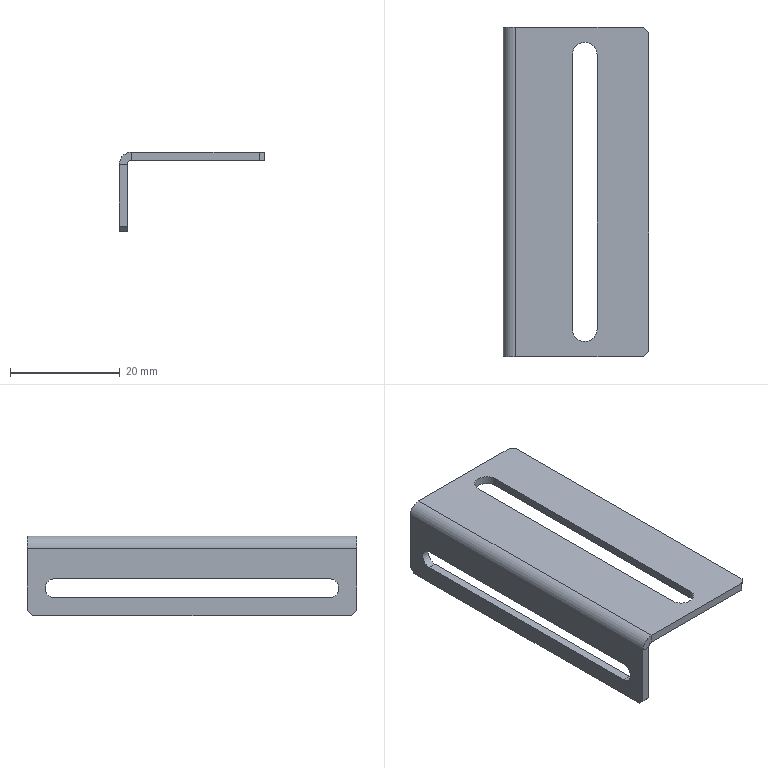Part | SolidWorks | features ICE 2, Chamfer 1, FlatPattern 1, SMBaseFlange 1, SheetMetal 1 | 1 solid | 26 faces | box 26.5 x 60 x 14.5 mm | volume 2856 mm3 | plane 20 | cylinder 6 | commonest cylinder face diameters 3.5 x2 4.5 x2 1.473 x1 4.473 x1
STEP:
#1=CARTESIAN_POINT('',(0.7366,60.,13.));
#2=VERTEX_POINT('',#1);
#3=CARTESIAN_POINT('',(0.7366,60.,14.5));
#4=VERTEX_POINT('',#3);
#5=CARTESIAN_POINT('',(0.7366,60.,13.));
#6=DIRECTION('',(0.,0.,1.));
#7=VECTOR('',#6,1000.);
#8=LINE('',#5,#7);
#9=EDGE_CURVE('',#2,#4,#8,.T.);
#10=ORIENTED_EDGE('',*,*,#9,.F.);
#11=CARTESIAN_POINT('',(0.,60.,12.263));
#12=VERTEX_POINT('',#11);
#13=CARTESIAN_POINT('',(0.7366,60.,12.263));
#14=DIRECTION('',(0.,1.,0.));
#15=DIRECTION('',(0.,0.,-1.));
#16=AXIS2_PLACEMENT_3D('',#13,#14,#15);
#17=CIRCLE('',#16,0.7366);
#18=EDGE_CURVE('',#12,#2,#17,.T.);
#19=ORIENTED_EDGE('',*,*,#18,.F.);
#20=CARTESIAN_POINT('',(-1.5,60.,12.263));
#21=VERTEX_POINT('',#20);
#22=CARTESIAN_POINT('',(-1.5,60.,12.263));
#23=DIRECTION('',(1.,0.,0.));
#24=VECTOR('',#23,1000.);
#25=LINE('',#22,#24);
#26=EDGE_CURVE('',#21,#12,#25,.T.);
#27=ORIENTED_EDGE('',*,*,#26,.F.);
#28=CARTESIAN_POINT('',(0.7366,60.,12.263));
#29=DIRECTION('',(0.,1.,0.));
#30=DIRECTION('',(1.,0.,0.));
#31=AXIS2_PLACEMENT_3D('',#28,#29,#30);
#32=CIRCLE('',#31,2.237);
#33=EDGE_CURVE('',#21,#4,#32,.T.);
#34=ORIENTED_EDGE('',*,*,#33,.T.);
#35=EDGE_LOOP('',(#10,#19,#27,#34));
#36=FACE_OUTER_BOUND('',#35,.T.);
#37=CARTESIAN_POINT('',(0.7366,60.,13.));
#38=DIRECTION('',(0.,1.,0.));
#39=DIRECTION('',(0.,0.,1.));
#40=AXIS2_PLACEMENT_3D('',#37,#38,#39);
#41=PLANE('',#40);
#42=ADVANCED_FACE('',(#36),#41,.T.);
#43=CARTESIAN_POINT('',(24.,60.,14.5));
#44=VERTEX_POINT('',#43);
#45=CARTESIAN_POINT('',(0.,60.,14.5));
#46=DIRECTION('',(1.,0.,0.));
#47=VECTOR('',#46,1000.);
#48=LINE('',#45,#47);
#49=EDGE_CURVE('',#4,#44,#48,.T.);
#50=ORIENTED_EDGE('',*,*,#49,.T.);
#51=CARTESIAN_POINT('',(24.,60.,13.));
#52=VERTEX_POINT('',#51);
#53=CARTESIAN_POINT('',(24.,60.,12.263));
#54=DIRECTION('',(0.,0.,-1.));
#55=VECTOR('',#54,1000.);
#56=LINE('',#53,#55);
#57=EDGE_CURVE('',#44,#52,#56,.T.);
#58=ORIENTED_EDGE('',*,*,#57,.T.);
#59=CARTESIAN_POINT('',(0.,60.,13.));
#60=DIRECTION('',(1.,0.,0.));
#61=VECTOR('',#60,1000.);
#62=LINE('',#59,#61);
#63=EDGE_CURVE('',#2,#52,#62,.T.);
#64=ORIENTED_EDGE('',*,*,#63,.F.);
#65=ORIENTED_EDGE('',*,*,#9,.T.);
#66=EDGE_LOOP('',(#50,#58,#64,#65));
#67=FACE_OUTER_BOUND('',#66,.T.);
#68=CARTESIAN_POINT('',(-1.5,60.,12.263));
#69=DIRECTION('',(0.,1.,0.));
#70=DIRECTION('',(0.,0.,1.));
#71=AXIS2_PLACEMENT_3D('',#68,#69,#70);
#72=PLANE('',#71);
#73=ADVANCED_FACE('',(#67),#72,.T.);
#74=CARTESIAN_POINT('',(0.,0.,12.263));
#75=VERTEX_POINT('',#74);
#76=CARTESIAN_POINT('',(-1.5,0.,12.263));
#77=VERTEX_POINT('',#76);
#78=CARTESIAN_POINT('',(0.,0.,12.263));
#79=DIRECTION('',(-1.,0.,0.));
#80=VECTOR('',#79,1000.);
#81=LINE('',#78,#80);
#82=EDGE_CURVE('',#75,#77,#81,.T.);
#83=ORIENTED_EDGE('',*,*,#82,.F.);
#84=CARTESIAN_POINT('',(0.7366,0.,13.));
#85=VERTEX_POINT('',#84);
#86=CARTESIAN_POINT('',(0.7366,0.,12.263));
#87=DIRECTION('',(0.,1.,0.));
#88=DIRECTION('',(0.,0.,-1.));
#89=AXIS2_PLACEMENT_3D('',#86,#87,#88);
#90=CIRCLE('',#89,0.7366);
#91=EDGE_CURVE('',#75,#85,#90,.T.);
#92=ORIENTED_EDGE('',*,*,#91,.T.);
#93=CARTESIAN_POINT('',(0.7366,0.,14.5));
#94=VERTEX_POINT('',#93);
#95=CARTESIAN_POINT('',(0.7366,0.,14.5));
#96=DIRECTION('',(0.,0.,-1.));
#97=VECTOR('',#96,1000.);
#98=LINE('',#95,#97);
#99=EDGE_CURVE('',#94,#85,#98,.T.);
#100=ORIENTED_EDGE('',*,*,#99,.F.);
#101=CARTESIAN_POINT('',(0.7366,0.,12.263));
#102=DIRECTION('',(0.,1.,0.));
#103=DIRECTION('',(1.,0.,0.));
#104=AXIS2_PLACEMENT_3D('',#101,#102,#103);
#105=CIRCLE('',#104,2.237);
#106=EDGE_CURVE('',#77,#94,#105,.T.);
#107=ORIENTED_EDGE('',*,*,#106,.F.);
#108=EDGE_LOOP('',(#83,#92,#100,#107));
#109=FACE_OUTER_BOUND('',#108,.T.);
#110=CARTESIAN_POINT('',(0.,0.,12.263));
#111=DIRECTION('',(0.,-1.,0.));
#112=DIRECTION('',(0.,0.,-1.));
#113=AXIS2_PLACEMENT_3D('',#110,#111,#112);
#114=PLANE('',#113);
#115=ADVANCED_FACE('',(#109),#114,.T.);
#116=CARTESIAN_POINT('',(-1.5,0.,1.));
#117=VERTEX_POINT('',#116);
#118=CARTESIAN_POINT('',(-1.5,0.,0.));
#119=DIRECTION('',(0.,0.,1.));
#120=VECTOR('',#119,1000.);
#121=LINE('',#118,#120);
#122=EDGE_CURVE('',#117,#77,#121,.T.);
#123=ORIENTED_EDGE('',*,*,#122,.F.);
#124=CARTESIAN_POINT('',(0.,0.,1.));
#125=VERTEX_POINT('',#124);
#126=CARTESIAN_POINT('',(0.7366,0.,1.));
#127=DIRECTION('',(1.,0.,0.));
#128=VECTOR('',#127,1000.);
#129=LINE('',#126,#128);
#130=EDGE_CURVE('',#117,#125,#129,.T.);
#131=ORIENTED_EDGE('',*,*,#130,.T.);
#132=CARTESIAN_POINT('',(0.,0.,0.));
#133=DIRECTION('',(0.,0.,1.));
#134=VECTOR('',#133,1000.);
#135=LINE('',#132,#134);
#136=EDGE_CURVE('',#125,#75,#135,.T.);
#137=ORIENTED_EDGE('',*,*,#136,.T.);
#138=ORIENTED_EDGE('',*,*,#82,.T.);
#139=EDGE_LOOP('',(#123,#131,#137,#138));
#140=FACE_OUTER_BOUND('',#139,.T.);
#141=CARTESIAN_POINT('',(0.7366,0.,14.5));
#142=DIRECTION('',(0.,-1.,0.));
#143=DIRECTION('',(0.,0.,-1.));
#144=AXIS2_PLACEMENT_3D('',#141,#142,#143);
#145=PLANE('',#144);
#146=ADVANCED_FACE('',(#140),#145,.T.);
#147=CARTESIAN_POINT('',(11.1,5.,14.5));
#148=VERTEX_POINT('',#147);
#149=CARTESIAN_POINT('',(11.1,55.,14.5));
#150=VERTEX_POINT('',#149);
#151=CARTESIAN_POINT('',(11.1,55.,14.5));
#152=DIRECTION('',(0.,1.,0.));
#153=VECTOR('',#152,1000.);
#154=LINE('',#151,#153);
#155=EDGE_CURVE('',#148,#150,#154,.T.);
#156=ORIENTED_EDGE('',*,*,#155,.T.);
#157=CARTESIAN_POINT('',(15.6,55.,14.5));
#158=VERTEX_POINT('',#157);
#159=CARTESIAN_POINT('',(13.35,55.,14.5));
#160=DIRECTION('',(0.,0.,-1.));
#161=DIRECTION('',(-1.,0.,0.));
#162=AXIS2_PLACEMENT_3D('',#159,#160,#161);
#163=CIRCLE('',#162,2.25);
#164=EDGE_CURVE('',#150,#158,#163,.T.);
#165=ORIENTED_EDGE('',*,*,#164,.T.);
#166=CARTESIAN_POINT('',(15.6,5.,14.5));
#167=VERTEX_POINT('',#166);
#168=CARTESIAN_POINT('',(15.6,55.,14.5));
#169=DIRECTION('',(0.,-1.,0.));
#170=VECTOR('',#169,1000.);
#171=LINE('',#168,#170);
#172=EDGE_CURVE('',#158,#167,#171,.T.);
#173=ORIENTED_EDGE('',*,*,#172,.T.);
#174=CARTESIAN_POINT('',(13.35,5.,14.5));
#175=DIRECTION('',(0.,0.,-1.));
#176=DIRECTION('',(-1.,0.,0.));
#177=AXIS2_PLACEMENT_3D('',#174,#175,#176);
#178=CIRCLE('',#177,2.25);
#179=EDGE_CURVE('',#167,#148,#178,.T.);
#180=ORIENTED_EDGE('',*,*,#179,.T.);
#181=EDGE_LOOP('',(#156,#165,#173,#180));
#182=FACE_BOUND('',#181,.T.);
#183=CARTESIAN_POINT('',(25.,59.,14.5));
#184=VERTEX_POINT('',#183);
#185=CARTESIAN_POINT('',(25.,1.,14.5));
#186=VERTEX_POINT('',#185);
#187=CARTESIAN_POINT('',(25.,60.,14.5));
#188=DIRECTION('',(0.,-1.,0.));
#189=VECTOR('',#188,1000.);
#190=LINE('',#187,#189);
#191=EDGE_CURVE('',#184,#186,#190,.T.);
#192=ORIENTED_EDGE('',*,*,#191,.F.);
#193=CARTESIAN_POINT('',(25.,59.,14.5));
#194=DIRECTION('',(-0.7071,0.7071,0.));
#195=VECTOR('',#194,1000.);
#196=LINE('',#193,#195);
#197=EDGE_CURVE('',#184,#44,#196,.T.);
#198=ORIENTED_EDGE('',*,*,#197,.T.);
#199=ORIENTED_EDGE('',*,*,#49,.F.);
#200=CARTESIAN_POINT('',(0.7366,60.,14.5));
#201=DIRECTION('',(0.,-1.,0.));
#202=VECTOR('',#201,1000.);
#203=LINE('',#200,#202);
#204=EDGE_CURVE('',#4,#94,#203,.T.);
#205=ORIENTED_EDGE('',*,*,#204,.T.);
#206=CARTESIAN_POINT('',(24.,0.,14.5));
#207=VERTEX_POINT('',#206);
#208=CARTESIAN_POINT('',(0.,0.,14.5));
#209=DIRECTION('',(1.,0.,0.));
#210=VECTOR('',#209,1000.);
#211=LINE('',#208,#210);
#212=EDGE_CURVE('',#94,#207,#211,.T.);
#213=ORIENTED_EDGE('',*,*,#212,.T.);
#214=CARTESIAN_POINT('',(24.,0.,14.5));
#215=DIRECTION('',(0.7071,0.7071,0.));
#216=VECTOR('',#215,1000.);
#217=LINE('',#214,#216);
#218=EDGE_CURVE('',#207,#186,#217,.T.);
#219=ORIENTED_EDGE('',*,*,#218,.T.);
#220=EDGE_LOOP('',(#192,#198,#199,#205,#213,#219));
#221=FACE_OUTER_BOUND('',#220,.T.);
#222=CARTESIAN_POINT('',(0.,60.,14.5));
#223=DIRECTION('',(0.,0.,-1.));
#224=DIRECTION('',(-1.,0.,0.));
#225=AXIS2_PLACEMENT_3D('',#222,#223,#224);
#226=PLANE('',#225);
#227=ADVANCED_FACE('',(#182,#221),#226,.F.);
#228=CARTESIAN_POINT('',(25.,59.,13.));
#229=VERTEX_POINT('',#228);
#230=CARTESIAN_POINT('',(25.,1.,13.));
#231=VERTEX_POINT('',#230);
#232=CARTESIAN_POINT('',(25.,60.,13.));
#233=DIRECTION('',(0.,-1.,0.));
#234=VECTOR('',#233,1000.);
#235=LINE('',#232,#234);
#236=EDGE_CURVE('',#229,#231,#235,.T.);
#237=ORIENTED_EDGE('',*,*,#236,.F.);
#238=CARTESIAN_POINT('',(25.,59.,13.));
#239=DIRECTION('',(0.,0.,1.));
#240=VECTOR('',#239,1000.);
#241=LINE('',#238,#240);
#242=EDGE_CURVE('',#229,#184,#241,.T.);
#243=ORIENTED_EDGE('',*,*,#242,.T.);
#244=ORIENTED_EDGE('',*,*,#191,.T.);
#245=CARTESIAN_POINT('',(25.,1.,13.));
#246=DIRECTION('',(0.,0.,-1.));
#247=VECTOR('',#246,1000.);
#248=LINE('',#245,#247);
#249=EDGE_CURVE('',#186,#231,#248,.T.);
#250=ORIENTED_EDGE('',*,*,#249,.T.);
#251=EDGE_LOOP('',(#237,#243,#244,#250));
#252=FACE_OUTER_BOUND('',#251,.T.);
#253=CARTESIAN_POINT('',(25.,60.,13.));
#254=DIRECTION('',(1.,0.,0.));
#255=DIRECTION('',(0.,0.,-1.));
#256=AXIS2_PLACEMENT_3D('',#253,#254,#255);
#257=PLANE('',#256);
#258=ADVANCED_FACE('',(#252),#257,.T.);
#259=CARTESIAN_POINT('',(11.1,55.,13.));
#260=VERTEX_POINT('',#259);
#261=CARTESIAN_POINT('',(15.6,55.,13.));
#262=VERTEX_POINT('',#261);
#263=CARTESIAN_POINT('',(13.35,55.,13.));
#264=DIRECTION('',(0.,0.,-1.));
#265=DIRECTION('',(-1.,0.,0.));
#266=AXIS2_PLACEMENT_3D('',#263,#264,#265);
#267=CIRCLE('',#266,2.25);
#268=EDGE_CURVE('',#260,#262,#267,.T.);
#269=ORIENTED_EDGE('',*,*,#268,.F.);
#270=CARTESIAN_POINT('',(11.1,5.,13.));
#271=VERTEX_POINT('',#270);
#272=CARTESIAN_POINT('',(11.1,55.,13.));
#273=DIRECTION('',(0.,1.,0.));
#274=VECTOR('',#273,1000.);
#275=LINE('',#272,#274);
#276=EDGE_CURVE('',#271,#260,#275,.T.);
#277=ORIENTED_EDGE('',*,*,#276,.F.);
#278=CARTESIAN_POINT('',(15.6,5.,13.));
#279=VERTEX_POINT('',#278);
#280=CARTESIAN_POINT('',(13.35,5.,13.));
#281=DIRECTION('',(0.,0.,-1.));
#282=DIRECTION('',(-1.,0.,0.));
#283=AXIS2_PLACEMENT_3D('',#280,#281,#282);
#284=CIRCLE('',#283,2.25);
#285=EDGE_CURVE('',#279,#271,#284,.T.);
#286=ORIENTED_EDGE('',*,*,#285,.F.);
#287=CARTESIAN_POINT('',(15.6,55.,13.));
#288=DIRECTION('',(0.,-1.,0.));
#289=VECTOR('',#288,1000.);
#290=LINE('',#287,#289);
#291=EDGE_CURVE('',#262,#279,#290,.T.);
#292=ORIENTED_EDGE('',*,*,#291,.F.);
#293=EDGE_LOOP('',(#269,#277,#286,#292));
#294=FACE_BOUND('',#293,.T.);
#295=ORIENTED_EDGE('',*,*,#63,.T.);
#296=CARTESIAN_POINT('',(12.,72.,13.));
#297=DIRECTION('',(0.7071,-0.7071,0.));
#298=VECTOR('',#297,1000.);
#299=LINE('',#296,#298);
#300=EDGE_CURVE('',#52,#229,#299,.T.);
#301=ORIENTED_EDGE('',*,*,#300,.T.);
#302=ORIENTED_EDGE('',*,*,#236,.T.);
#303=CARTESIAN_POINT('',(24.,0.,13.));
#304=VERTEX_POINT('',#303);
#305=CARTESIAN_POINT('',(42.,18.,13.));
#306=DIRECTION('',(-0.7071,-0.7071,0.));
#307=VECTOR('',#306,1000.);
#308=LINE('',#305,#307);
#309=EDGE_CURVE('',#231,#304,#308,.T.);
#310=ORIENTED_EDGE('',*,*,#309,.T.);
#311=CARTESIAN_POINT('',(0.,0.,13.));
#312=DIRECTION('',(1.,0.,0.));
#313=VECTOR('',#312,1000.);
#314=LINE('',#311,#313);
#315=EDGE_CURVE('',#85,#304,#314,.T.);
#316=ORIENTED_EDGE('',*,*,#315,.F.);
#317=CARTESIAN_POINT('',(0.7366,60.,13.));
#318=DIRECTION('',(0.,-1.,0.));
#319=VECTOR('',#318,1000.);
#320=LINE('',#317,#319);
#321=EDGE_CURVE('',#2,#85,#320,.T.);
#322=ORIENTED_EDGE('',*,*,#321,.F.);
#323=EDGE_LOOP('',(#295,#301,#302,#310,#316,#322));
#324=FACE_OUTER_BOUND('',#323,.T.);
#325=CARTESIAN_POINT('',(0.,60.,13.));
#326=DIRECTION('',(0.,0.,-1.));
#327=DIRECTION('',(-1.,0.,0.));
#328=AXIS2_PLACEMENT_3D('',#325,#326,#327);
#329=PLANE('',#328);
#330=ADVANCED_FACE('',(#294,#324),#329,.T.);
#331=ORIENTED_EDGE('',*,*,#91,.F.);
#332=CARTESIAN_POINT('',(0.,60.,12.263));
#333=DIRECTION('',(0.,-1.,0.));
#334=VECTOR('',#333,1000.);
#335=LINE('',#332,#334);
#336=EDGE_CURVE('',#12,#75,#335,.T.);
#337=ORIENTED_EDGE('',*,*,#336,.F.);
#338=ORIENTED_EDGE('',*,*,#18,.T.);
#339=ORIENTED_EDGE('',*,*,#321,.T.);
#340=EDGE_LOOP('',(#331,#337,#338,#339));
#341=FACE_OUTER_BOUND('',#340,.T.);
#342=CARTESIAN_POINT('',(0.7366,60.,12.263));
#343=DIRECTION('',(0.,-1.,0.));
#344=DIRECTION('',(0.,0.,-1.));
#345=AXIS2_PLACEMENT_3D('',#342,#343,#344);
#346=CYLINDRICAL_SURFACE('',#345,0.7366);
#347=ADVANCED_FACE('',(#341),#346,.F.);
#348=CARTESIAN_POINT('',(0.,55.,3.25));
#349=VERTEX_POINT('',#348);
#350=CARTESIAN_POINT('',(0.,55.,6.75));
#351=VERTEX_POINT('',#350);
#352=CARTESIAN_POINT('',(0.,55.,5.));
#353=DIRECTION('',(1.,0.,0.));
#354=DIRECTION('',(0.,0.,-1.));
#355=AXIS2_PLACEMENT_3D('',#352,#353,#354);
#356=CIRCLE('',#355,1.75);
#357=EDGE_CURVE('',#349,#351,#356,.T.);
#358=ORIENTED_EDGE('',*,*,#357,.F.);
#359=CARTESIAN_POINT('',(0.,5.,3.25));
#360=VERTEX_POINT('',#359);
#361=CARTESIAN_POINT('',(0.,55.,3.25));
#362=DIRECTION('',(0.,1.,0.));
#363=VECTOR('',#362,1000.);
#364=LINE('',#361,#363);
#365=EDGE_CURVE('',#360,#349,#364,.T.);
#366=ORIENTED_EDGE('',*,*,#365,.F.);
#367=CARTESIAN_POINT('',(0.,5.,6.75));
#368=VERTEX_POINT('',#367);
#369=CARTESIAN_POINT('',(0.,5.,5.));
#370=DIRECTION('',(1.,0.,0.));
#371=DIRECTION('',(0.,0.,-1.));
#372=AXIS2_PLACEMENT_3D('',#369,#370,#371);
#373=CIRCLE('',#372,1.75);
#374=EDGE_CURVE('',#368,#360,#373,.T.);
#375=ORIENTED_EDGE('',*,*,#374,.F.);
#376=CARTESIAN_POINT('',(0.,55.,6.75));
#377=DIRECTION('',(0.,-1.,0.));
#378=VECTOR('',#377,1000.);
#379=LINE('',#376,#378);
#380=EDGE_CURVE('',#351,#368,#379,.T.);
#381=ORIENTED_EDGE('',*,*,#380,.F.);
#382=EDGE_LOOP('',(#358,#366,#375,#381));
#383=FACE_BOUND('',#382,.T.);
#384=ORIENTED_EDGE('',*,*,#136,.F.);
#385=CARTESIAN_POINT('',(0.,1.,0.));
#386=VERTEX_POINT('',#385);
#387=CARTESIAN_POINT('',(0.,30.5,-29.5));
#388=DIRECTION('',(0.,0.7071,-0.7071));
#389=VECTOR('',#388,1000.);
#390=LINE('',#387,#389);
#391=EDGE_CURVE('',#125,#386,#390,.T.);
#392=ORIENTED_EDGE('',*,*,#391,.T.);
#393=CARTESIAN_POINT('',(0.,59.,0.));
#394=VERTEX_POINT('',#393);
#395=CARTESIAN_POINT('',(0.,60.,0.));
#396=DIRECTION('',(0.,-1.,0.));
#397=VECTOR('',#396,1000.);
#398=LINE('',#395,#397);
#399=EDGE_CURVE('',#394,#386,#398,.T.);
#400=ORIENTED_EDGE('',*,*,#399,.F.);
#401=CARTESIAN_POINT('',(0.,60.,1.));
#402=VERTEX_POINT('',#401);
#403=CARTESIAN_POINT('',(0.,59.5,0.5));
#404=DIRECTION('',(0.,0.7071,0.7071));
#405=VECTOR('',#404,1000.);
#406=LINE('',#403,#405);
#407=EDGE_CURVE('',#394,#402,#406,.T.);
#408=ORIENTED_EDGE('',*,*,#407,.T.);
#409=CARTESIAN_POINT('',(0.,60.,0.));
#410=DIRECTION('',(0.,0.,1.));
#411=VECTOR('',#410,1000.);
#412=LINE('',#409,#411);
#413=EDGE_CURVE('',#402,#12,#412,.T.);
#414=ORIENTED_EDGE('',*,*,#413,.T.);
#415=ORIENTED_EDGE('',*,*,#336,.T.);
#416=EDGE_LOOP('',(#384,#392,#400,#408,#414,#415));
#417=FACE_OUTER_BOUND('',#416,.T.);
#418=CARTESIAN_POINT('',(0.,60.,0.));
#419=DIRECTION('',(1.,0.,0.));
#420=DIRECTION('',(0.,0.,-1.));
#421=AXIS2_PLACEMENT_3D('',#418,#419,#420);
#422=PLANE('',#421);
#423=ADVANCED_FACE('',(#383,#417),#422,.T.);
#424=ORIENTED_EDGE('',*,*,#399,.T.);
#425=CARTESIAN_POINT('',(-1.5,1.,0.));
#426=VERTEX_POINT('',#425);
#427=CARTESIAN_POINT('',(-1.5,1.,0.));
#428=DIRECTION('',(-1.,0.,0.));
#429=VECTOR('',#428,1000.);
#430=LINE('',#427,#429);
#431=EDGE_CURVE('',#386,#426,#430,.T.);
#432=ORIENTED_EDGE('',*,*,#431,.T.);
#433=CARTESIAN_POINT('',(-1.5,59.,0.));
#434=VERTEX_POINT('',#433);
#435=CARTESIAN_POINT('',(-1.5,60.,0.));
#436=DIRECTION('',(0.,-1.,0.));
#437=VECTOR('',#436,1000.);
#438=LINE('',#435,#437);
#439=EDGE_CURVE('',#434,#426,#438,.T.);
#440=ORIENTED_EDGE('',*,*,#439,.F.);
#441=CARTESIAN_POINT('',(0.,59.,0.));
#442=DIRECTION('',(1.,0.,0.));
#443=VECTOR('',#442,1000.);
#444=LINE('',#441,#443);
#445=EDGE_CURVE('',#434,#394,#444,.T.);
#446=ORIENTED_EDGE('',*,*,#445,.T.);
#447=EDGE_LOOP('',(#424,#432,#440,#446));
#448=FACE_OUTER_BOUND('',#447,.T.);
#449=CARTESIAN_POINT('',(-1.5,60.,0.));
#450=DIRECTION('',(0.,0.,-1.));
#451=DIRECTION('',(-1.,0.,0.));
#452=AXIS2_PLACEMENT_3D('',#449,#450,#451);
#453=PLANE('',#452);
#454=ADVANCED_FACE('',(#448),#453,.T.);
#455=CARTESIAN_POINT('',(-1.5,5.,3.25));
#456=VERTEX_POINT('',#455);
#457=CARTESIAN_POINT('',(-1.5,55.,3.25));
#458=VERTEX_POINT('',#457);
#459=CARTESIAN_POINT('',(-1.5,55.,3.25));
#460=DIRECTION('',(0.,1.,0.));
#461=VECTOR('',#460,1000.);
#462=LINE('',#459,#461);
#463=EDGE_CURVE('',#456,#458,#462,.T.);
#464=ORIENTED_EDGE('',*,*,#463,.T.);
#465=CARTESIAN_POINT('',(-1.5,55.,6.75));
#466=VERTEX_POINT('',#465);
#467=CARTESIAN_POINT('',(-1.5,55.,5.));
#468=DIRECTION('',(1.,0.,0.));
#469=DIRECTION('',(0.,0.,-1.));
#470=AXIS2_PLACEMENT_3D('',#467,#468,#469);
#471=CIRCLE('',#470,1.75);
#472=EDGE_CURVE('',#458,#466,#471,.T.);
#473=ORIENTED_EDGE('',*,*,#472,.T.);
#474=CARTESIAN_POINT('',(-1.5,5.,6.75));
#475=VERTEX_POINT('',#474);
#476=CARTESIAN_POINT('',(-1.5,55.,6.75));
#477=DIRECTION('',(0.,-1.,0.));
#478=VECTOR('',#477,1000.);
#479=LINE('',#476,#478);
#480=EDGE_CURVE('',#466,#475,#479,.T.);
#481=ORIENTED_EDGE('',*,*,#480,.T.);
#482=CARTESIAN_POINT('',(-1.5,5.,5.));
#483=DIRECTION('',(1.,0.,0.));
#484=DIRECTION('',(0.,0.,-1.));
#485=AXIS2_PLACEMENT_3D('',#482,#483,#484);
#486=CIRCLE('',#485,1.75);
#487=EDGE_CURVE('',#475,#456,#486,.T.);
#488=ORIENTED_EDGE('',*,*,#487,.T.);
#489=EDGE_LOOP('',(#464,#473,#481,#488));
#490=FACE_BOUND('',#489,.T.);
#491=ORIENTED_EDGE('',*,*,#439,.T.);
#492=CARTESIAN_POINT('',(-1.5,0.,1.));
#493=DIRECTION('',(0.,-0.7071,0.7071));
#494=VECTOR('',#493,1000.);
#495=LINE('',#492,#494);
#496=EDGE_CURVE('',#426,#117,#495,.T.);
#497=ORIENTED_EDGE('',*,*,#496,.T.);
#498=ORIENTED_EDGE('',*,*,#122,.T.);
#499=CARTESIAN_POINT('',(-1.5,60.,12.263));
#500=DIRECTION('',(0.,-1.,0.));
#501=VECTOR('',#500,1000.);
#502=LINE('',#499,#501);
#503=EDGE_CURVE('',#21,#77,#502,.T.);
#504=ORIENTED_EDGE('',*,*,#503,.F.);
#505=CARTESIAN_POINT('',(-1.5,60.,1.));
#506=VERTEX_POINT('',#505);
#507=CARTESIAN_POINT('',(-1.5,60.,0.));
#508=DIRECTION('',(0.,0.,1.));
#509=VECTOR('',#508,1000.);
#510=LINE('',#507,#509);
#511=EDGE_CURVE('',#506,#21,#510,.T.);
#512=ORIENTED_EDGE('',*,*,#511,.F.);
#513=CARTESIAN_POINT('',(-1.5,59.,0.));
#514=DIRECTION('',(0.,-0.7071,-0.7071));
#515=VECTOR('',#514,1000.);
#516=LINE('',#513,#515);
#517=EDGE_CURVE('',#506,#434,#516,.T.);
#518=ORIENTED_EDGE('',*,*,#517,.T.);
#519=EDGE_LOOP('',(#491,#497,#498,#504,#512,#518));
#520=FACE_OUTER_BOUND('',#519,.T.);
#521=CARTESIAN_POINT('',(-1.5,60.,0.));
#522=DIRECTION('',(1.,0.,0.));
#523=DIRECTION('',(0.,0.,-1.));
#524=AXIS2_PLACEMENT_3D('',#521,#522,#523);
#525=PLANE('',#524);
#526=ADVANCED_FACE('',(#490,#520),#525,.F.);
#527=ORIENTED_EDGE('',*,*,#106,.T.);
#528=ORIENTED_EDGE('',*,*,#204,.F.);
#529=ORIENTED_EDGE('',*,*,#33,.F.);
#530=ORIENTED_EDGE('',*,*,#503,.T.);
#531=EDGE_LOOP('',(#527,#528,#529,#530));
#532=FACE_OUTER_BOUND('',#531,.T.);
#533=CARTESIAN_POINT('',(0.7366,60.,12.263));
#534=DIRECTION('',(0.,-1.,0.));
#535=DIRECTION('',(0.,0.,-1.));
#536=AXIS2_PLACEMENT_3D('',#533,#534,#535);
#537=CYLINDRICAL_SURFACE('',#536,2.237);
#538=ADVANCED_FACE('',(#532),#537,.T.);
#539=ORIENTED_EDGE('',*,*,#413,.F.);
#540=CARTESIAN_POINT('',(-1.5,60.,1.));
#541=DIRECTION('',(-1.,0.,0.));
#542=VECTOR('',#541,1000.);
#543=LINE('',#540,#542);
#544=EDGE_CURVE('',#402,#506,#543,.T.);
#545=ORIENTED_EDGE('',*,*,#544,.T.);
#546=ORIENTED_EDGE('',*,*,#511,.T.);
#547=ORIENTED_EDGE('',*,*,#26,.T.);
#548=EDGE_LOOP('',(#539,#545,#546,#547));
#549=FACE_OUTER_BOUND('',#548,.T.);
#550=CARTESIAN_POINT('',(0.7366,60.,12.263));
#551=DIRECTION('',(0.,-1.,0.));
#552=DIRECTION('',(-1.,0.,0.));
#553=AXIS2_PLACEMENT_3D('',#550,#551,#552);
#554=PLANE('',#553);
#555=ADVANCED_FACE('',(#549),#554,.F.);
#556=ORIENTED_EDGE('',*,*,#315,.T.);
#557=CARTESIAN_POINT('',(24.,0.,12.263));
#558=DIRECTION('',(0.,0.,1.));
#559=VECTOR('',#558,1000.);
#560=LINE('',#557,#559);
#561=EDGE_CURVE('',#304,#207,#560,.T.);
#562=ORIENTED_EDGE('',*,*,#561,.T.);
#563=ORIENTED_EDGE('',*,*,#212,.F.);
#564=ORIENTED_EDGE('',*,*,#99,.T.);
#565=EDGE_LOOP('',(#556,#562,#563,#564));
#566=FACE_OUTER_BOUND('',#565,.T.);
#567=CARTESIAN_POINT('',(0.7366,0.,12.263));
#568=DIRECTION('',(0.,-1.,0.));
#569=DIRECTION('',(-1.,0.,0.));
#570=AXIS2_PLACEMENT_3D('',#567,#568,#569);
#571=PLANE('',#570);
#572=ADVANCED_FACE('',(#566),#571,.T.);
#573=ORIENTED_EDGE('',*,*,#357,.T.);
#574=CARTESIAN_POINT('',(-1.5,55.,6.75));
#575=DIRECTION('',(1.,0.,0.));
#576=VECTOR('',#575,1000.);
#577=LINE('',#574,#576);
#578=EDGE_CURVE('',#466,#351,#577,.T.);
#579=ORIENTED_EDGE('',*,*,#578,.F.);
#580=ORIENTED_EDGE('',*,*,#472,.F.);
#581=CARTESIAN_POINT('',(-1.5,55.,3.25));
#582=DIRECTION('',(1.,0.,0.));
#583=VECTOR('',#582,1000.);
#584=LINE('',#581,#583);
#585=EDGE_CURVE('',#458,#349,#584,.T.);
#586=ORIENTED_EDGE('',*,*,#585,.T.);
#587=EDGE_LOOP('',(#573,#579,#580,#586));
#588=FACE_OUTER_BOUND('',#587,.T.);
#589=CARTESIAN_POINT('',(-1.5,55.,5.));
#590=DIRECTION('',(1.,0.,0.));
#591=DIRECTION('',(0.,0.,-1.));
#592=AXIS2_PLACEMENT_3D('',#589,#590,#591);
#593=CYLINDRICAL_SURFACE('',#592,1.75);
#594=ADVANCED_FACE('',(#588),#593,.F.);
#595=ORIENTED_EDGE('',*,*,#365,.T.);
#596=ORIENTED_EDGE('',*,*,#585,.F.);
#597=ORIENTED_EDGE('',*,*,#463,.F.);
#598=CARTESIAN_POINT('',(-1.5,5.,3.25));
#599=DIRECTION('',(1.,0.,0.));
#600=VECTOR('',#599,1000.);
#601=LINE('',#598,#600);
#602=EDGE_CURVE('',#456,#360,#601,.T.);
#603=ORIENTED_EDGE('',*,*,#602,.T.);
#604=EDGE_LOOP('',(#595,#596,#597,#603));
#605=FACE_OUTER_BOUND('',#604,.T.);
#606=CARTESIAN_POINT('',(-1.5,55.,3.25));
#607=DIRECTION('',(0.,0.,-1.));
#608=DIRECTION('',(-1.,0.,0.));
#609=AXIS2_PLACEMENT_3D('',#606,#607,#608);
#610=PLANE('',#609);
#611=ADVANCED_FACE('',(#605),#610,.F.);
#612=ORIENTED_EDGE('',*,*,#374,.T.);
#613=ORIENTED_EDGE('',*,*,#602,.F.);
#614=ORIENTED_EDGE('',*,*,#487,.F.);
#615=CARTESIAN_POINT('',(-1.5,5.,6.75));
#616=DIRECTION('',(1.,0.,0.));
#617=VECTOR('',#616,1000.);
#618=LINE('',#615,#617);
#619=EDGE_CURVE('',#475,#368,#618,.T.);
#620=ORIENTED_EDGE('',*,*,#619,.T.);
#621=EDGE_LOOP('',(#612,#613,#614,#620));
#622=FACE_OUTER_BOUND('',#621,.T.);
#623=CARTESIAN_POINT('',(-1.5,5.,5.));
#624=DIRECTION('',(1.,0.,0.));
#625=DIRECTION('',(0.,0.,-1.));
#626=AXIS2_PLACEMENT_3D('',#623,#624,#625);
#627=CYLINDRICAL_SURFACE('',#626,1.75);
#628=ADVANCED_FACE('',(#622),#627,.F.);
#629=ORIENTED_EDGE('',*,*,#380,.T.);
#630=ORIENTED_EDGE('',*,*,#619,.F.);
#631=ORIENTED_EDGE('',*,*,#480,.F.);
#632=ORIENTED_EDGE('',*,*,#578,.T.);
#633=EDGE_LOOP('',(#629,#630,#631,#632));
#634=FACE_OUTER_BOUND('',#633,.T.);
#635=CARTESIAN_POINT('',(-1.5,55.,6.75));
#636=DIRECTION('',(0.,0.,1.));
#637=DIRECTION('',(1.,0.,0.));
#638=AXIS2_PLACEMENT_3D('',#635,#636,#637);
#639=PLANE('',#638);
#640=ADVANCED_FACE('',(#634),#639,.F.);
#641=ORIENTED_EDGE('',*,*,#300,.F.);
#642=ORIENTED_EDGE('',*,*,#57,.F.);
#643=ORIENTED_EDGE('',*,*,#197,.F.);
#644=ORIENTED_EDGE('',*,*,#242,.F.);
#645=EDGE_LOOP('',(#641,#642,#643,#644));
#646=FACE_OUTER_BOUND('',#645,.T.);
#647=CARTESIAN_POINT('',(25.,59.,13.));
#648=DIRECTION('',(-0.7071,-0.7071,0.));
#649=DIRECTION('',(0.,0.,1.));
#650=AXIS2_PLACEMENT_3D('',#647,#648,#649);
#651=PLANE('',#650);
#652=ADVANCED_FACE('',(#646),#651,.F.);
#653=ORIENTED_EDGE('',*,*,#309,.F.);
#654=ORIENTED_EDGE('',*,*,#249,.F.);
#655=ORIENTED_EDGE('',*,*,#218,.F.);
#656=ORIENTED_EDGE('',*,*,#561,.F.);
#657=EDGE_LOOP('',(#653,#654,#655,#656));
#658=FACE_OUTER_BOUND('',#657,.T.);
#659=CARTESIAN_POINT('',(24.,0.,12.263));
#660=DIRECTION('',(-0.7071,0.7071,0.));
#661=DIRECTION('',(0.,0.,1.));
#662=AXIS2_PLACEMENT_3D('',#659,#660,#661);
#663=PLANE('',#662);
#664=ADVANCED_FACE('',(#658),#663,.F.);
#665=ORIENTED_EDGE('',*,*,#496,.F.);
#666=ORIENTED_EDGE('',*,*,#431,.F.);
#667=ORIENTED_EDGE('',*,*,#391,.F.);
#668=ORIENTED_EDGE('',*,*,#130,.F.);
#669=EDGE_LOOP('',(#665,#666,#667,#668));
#670=FACE_OUTER_BOUND('',#669,.T.);
#671=CARTESIAN_POINT('',(0.7366,0.,1.));
#672=DIRECTION('',(0.,0.7071,0.7071));
#673=DIRECTION('',(1.,0.,0.));
#674=AXIS2_PLACEMENT_3D('',#671,#672,#673);
#675=PLANE('',#674);
#676=ADVANCED_FACE('',(#670),#675,.F.);
#677=ORIENTED_EDGE('',*,*,#517,.F.);
#678=ORIENTED_EDGE('',*,*,#544,.F.);
#679=ORIENTED_EDGE('',*,*,#407,.F.);
#680=ORIENTED_EDGE('',*,*,#445,.F.);
#681=EDGE_LOOP('',(#677,#678,#679,#680));
#682=FACE_OUTER_BOUND('',#681,.T.);
#683=CARTESIAN_POINT('',(-1.5,59.,0.));
#684=DIRECTION('',(0.,0.7071,-0.7071));
#685=DIRECTION('',(-1.,0.,0.));
#686=AXIS2_PLACEMENT_3D('',#683,#684,#685);
#687=PLANE('',#686);
#688=ADVANCED_FACE('',(#682),#687,.T.);
#689=ORIENTED_EDGE('',*,*,#268,.T.);
#690=CARTESIAN_POINT('',(15.6,55.,14.5));
#691=DIRECTION('',(0.,0.,-1.));
#692=VECTOR('',#691,1000.);
#693=LINE('',#690,#692);
#694=EDGE_CURVE('',#158,#262,#693,.T.);
#695=ORIENTED_EDGE('',*,*,#694,.F.);
#696=ORIENTED_EDGE('',*,*,#164,.F.);
#697=CARTESIAN_POINT('',(11.1,55.,14.5));
#698=DIRECTION('',(0.,0.,-1.));
#699=VECTOR('',#698,1000.);
#700=LINE('',#697,#699);
#701=EDGE_CURVE('',#150,#260,#700,.T.);
#702=ORIENTED_EDGE('',*,*,#701,.T.);
#703=EDGE_LOOP('',(#689,#695,#696,#702));
#704=FACE_OUTER_BOUND('',#703,.T.);
#705=CARTESIAN_POINT('',(13.35,55.,14.5));
#706=DIRECTION('',(0.,0.,-1.));
#707=DIRECTION('',(-1.,0.,0.));
#708=AXIS2_PLACEMENT_3D('',#705,#706,#707);
#709=CYLINDRICAL_SURFACE('',#708,2.25);
#710=ADVANCED_FACE('',(#704),#709,.F.);
#711=ORIENTED_EDGE('',*,*,#276,.T.);
#712=ORIENTED_EDGE('',*,*,#701,.F.);
#713=ORIENTED_EDGE('',*,*,#155,.F.);
#714=CARTESIAN_POINT('',(11.1,5.,14.5));
#715=DIRECTION('',(0.,0.,-1.));
#716=VECTOR('',#715,1000.);
#717=LINE('',#714,#716);
#718=EDGE_CURVE('',#148,#271,#717,.T.);
#719=ORIENTED_EDGE('',*,*,#718,.T.);
#720=EDGE_LOOP('',(#711,#712,#713,#719));
#721=FACE_OUTER_BOUND('',#720,.T.);
#722=CARTESIAN_POINT('',(11.1,55.,14.5));
#723=DIRECTION('',(-1.,0.,0.));
#724=DIRECTION('',(0.,-1.,0.));
#725=AXIS2_PLACEMENT_3D('',#722,#723,#724);
#726=PLANE('',#725);
#727=ADVANCED_FACE('',(#721),#726,.F.);
#728=ORIENTED_EDGE('',*,*,#285,.T.);
#729=ORIENTED_EDGE('',*,*,#718,.F.);
#730=ORIENTED_EDGE('',*,*,#179,.F.);
#731=CARTESIAN_POINT('',(15.6,5.,14.5));
#732=DIRECTION('',(0.,0.,-1.));
#733=VECTOR('',#732,1000.);
#734=LINE('',#731,#733);
#735=EDGE_CURVE('',#167,#279,#734,.T.);
#736=ORIENTED_EDGE('',*,*,#735,.T.);
#737=EDGE_LOOP('',(#728,#729,#730,#736));
#738=FACE_OUTER_BOUND('',#737,.T.);
#739=CARTESIAN_POINT('',(13.35,5.,14.5));
#740=DIRECTION('',(0.,0.,-1.));
#741=DIRECTION('',(-1.,0.,0.));
#742=AXIS2_PLACEMENT_3D('',#739,#740,#741);
#743=CYLINDRICAL_SURFACE('',#742,2.25);
#744=ADVANCED_FACE('',(#738),#743,.F.);
#745=ORIENTED_EDGE('',*,*,#291,.T.);
#746=ORIENTED_EDGE('',*,*,#735,.F.);
#747=ORIENTED_EDGE('',*,*,#172,.F.);
#748=ORIENTED_EDGE('',*,*,#694,.T.);
#749=EDGE_LOOP('',(#745,#746,#747,#748));
#750=FACE_OUTER_BOUND('',#749,.T.);
#751=CARTESIAN_POINT('',(15.6,55.,14.5));
#752=DIRECTION('',(1.,0.,0.));
#753=DIRECTION('',(0.,1.,0.));
#754=AXIS2_PLACEMENT_3D('',#751,#752,#753);
#755=PLANE('',#754);
#756=ADVANCED_FACE('',(#750),#755,.F.);
#757=CLOSED_SHELL('',(#42,#73,#115,#146,#227,#258,#330,#347,#423,#454,#526,#538,#555,#572,#594,#611,#628,#640,#652,#664,#676,#688,#710,#727,#744,#756));
#758=MANIFOLD_SOLID_BREP('',#757);
#759=CARTESIAN_POINT('',(0.,0.,0.));
#760=DIRECTION('',(0.,0.,1.));
#761=DIRECTION('',(1.,0.,0.));
#762=AXIS2_PLACEMENT_3D('',#759,#760,#761);
#763=(LENGTH_UNIT()NAMED_UNIT(*)SI_UNIT(.MILLI.,.METRE.));
#764=UNCERTAINTY_MEASURE_WITH_UNIT(LENGTH_MEASURE(0.00001),#763,'','');
#765=(NAMED_UNIT(*)PLANE_ANGLE_UNIT()SI_UNIT($,.RADIAN.));
#766=(NAMED_UNIT(*)SI_UNIT($,.STERADIAN.)SOLID_ANGLE_UNIT());
#767=(GEOMETRIC_REPRESENTATION_CONTEXT(3)GLOBAL_UNCERTAINTY_ASSIGNED_CONTEXT((#764))GLOBAL_UNIT_ASSIGNED_CONTEXT((#763,#765,#766))REPRESENTATION_CONTEXT('',''));
#768=ADVANCED_BREP_SHAPE_REPRESENTATION('',(#758,#762),#767);